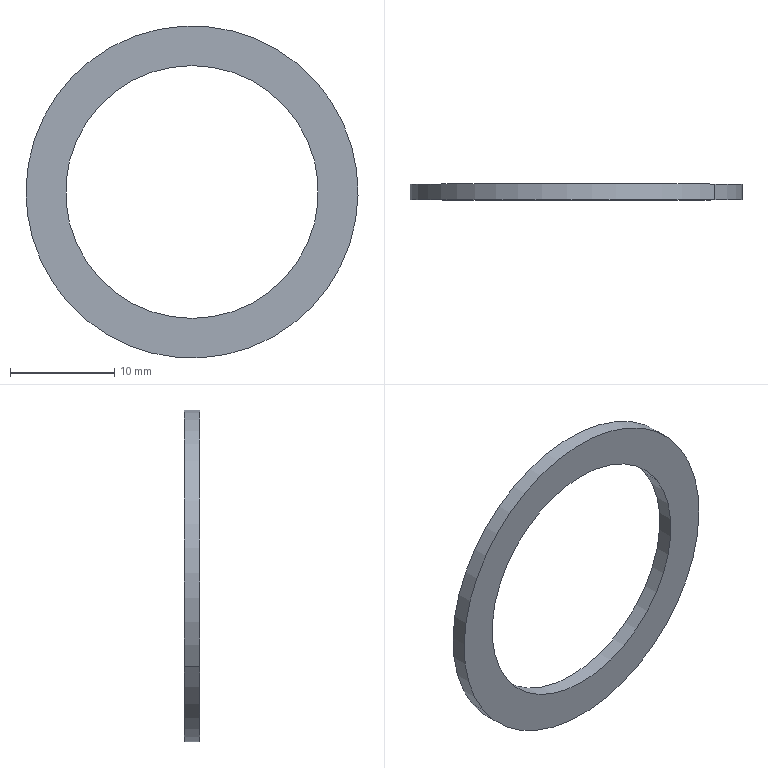Part | SolidWorks | features BaseBody 1 | 1 solid | 6 faces | box 31.8 x 1.5 x 31.8 mm | volume 501.398 mm3 | cylinder 4 | plane 2 | commonest cylinder face diameters 24.2 x2 31.8 x2
STEP:
#1=CARTESIAN_POINT('',(196.311,-137.,298.196));
#2=VERTEX_POINT('',#1);
#3=CARTESIAN_POINT('',(169.689,-137.,280.804));
#4=VERTEX_POINT('',#3);
#5=CARTESIAN_POINT('',(183.,-137.,289.5));
#6=DIRECTION('',(0.,-1.,0.));
#7=DIRECTION('',(0.,0.,1.));
#8=AXIS2_PLACEMENT_3D('',#5,#6,#7);
#9=CIRCLE('',#8,15.9);
#10=EDGE_CURVE('',#2,#4,#9,.T.);
#11=ORIENTED_EDGE('',*,*,#10,.F.);
#12=CARTESIAN_POINT('',(196.311,-135.5,298.196));
#13=VERTEX_POINT('',#12);
#14=CARTESIAN_POINT('',(196.311,-137.,298.196));
#15=DIRECTION('',(0.,1.,0.));
#16=VECTOR('',#15,1000.);
#17=LINE('',#14,#16);
#18=EDGE_CURVE('',#2,#13,#17,.T.);
#19=ORIENTED_EDGE('',*,*,#18,.T.);
#20=CARTESIAN_POINT('',(169.689,-135.5,280.804));
#21=VERTEX_POINT('',#20);
#22=CARTESIAN_POINT('',(183.,-135.5,289.5));
#23=DIRECTION('',(0.,1.,0.));
#24=DIRECTION('',(0.,0.,1.));
#25=AXIS2_PLACEMENT_3D('',#22,#23,#24);
#26=CIRCLE('',#25,15.9);
#27=EDGE_CURVE('',#21,#13,#26,.T.);
#28=ORIENTED_EDGE('',*,*,#27,.F.);
#29=CARTESIAN_POINT('',(169.689,-137.,280.804));
#30=DIRECTION('',(0.,1.,0.));
#31=VECTOR('',#30,1000.);
#32=LINE('',#29,#31);
#33=EDGE_CURVE('',#4,#21,#32,.T.);
#34=ORIENTED_EDGE('',*,*,#33,.F.);
#35=EDGE_LOOP('',(#11,#19,#28,#34));
#36=FACE_OUTER_BOUND('',#35,.T.);
#37=CARTESIAN_POINT('',(183.,-137.,289.5));
#38=DIRECTION('',(0.,1.,0.));
#39=DIRECTION('',(-0.8372,0.,-0.5469));
#40=AXIS2_PLACEMENT_3D('',#37,#38,#39);
#41=CYLINDRICAL_SURFACE('',#40,15.9);
#42=ADVANCED_FACE('',(#36),#41,.T.);
#43=CARTESIAN_POINT('',(172.87,-137.,282.882));
#44=VERTEX_POINT('',#43);
#45=CARTESIAN_POINT('',(193.13,-137.,296.118));
#46=VERTEX_POINT('',#45);
#47=CARTESIAN_POINT('',(183.,-137.,289.5));
#48=DIRECTION('',(0.,-1.,0.));
#49=DIRECTION('',(0.,0.,1.));
#50=AXIS2_PLACEMENT_3D('',#47,#48,#49);
#51=CIRCLE('',#50,12.1);
#52=EDGE_CURVE('',#44,#46,#51,.T.);
#53=ORIENTED_EDGE('',*,*,#52,.T.);
#54=CARTESIAN_POINT('',(193.13,-135.5,296.118));
#55=VERTEX_POINT('',#54);
#56=CARTESIAN_POINT('',(193.13,-137.,296.118));
#57=DIRECTION('',(0.,1.,0.));
#58=VECTOR('',#57,1000.);
#59=LINE('',#56,#58);
#60=EDGE_CURVE('',#46,#55,#59,.T.);
#61=ORIENTED_EDGE('',*,*,#60,.T.);
#62=CARTESIAN_POINT('',(172.87,-135.5,282.882));
#63=VERTEX_POINT('',#62);
#64=CARTESIAN_POINT('',(183.,-135.5,289.5));
#65=DIRECTION('',(0.,-1.,0.));
#66=DIRECTION('',(0.,0.,1.));
#67=AXIS2_PLACEMENT_3D('',#64,#65,#66);
#68=CIRCLE('',#67,12.1);
#69=EDGE_CURVE('',#63,#55,#68,.T.);
#70=ORIENTED_EDGE('',*,*,#69,.F.);
#71=CARTESIAN_POINT('',(172.87,-137.,282.882));
#72=DIRECTION('',(0.,1.,0.));
#73=VECTOR('',#72,1000.);
#74=LINE('',#71,#73);
#75=EDGE_CURVE('',#44,#63,#74,.T.);
#76=ORIENTED_EDGE('',*,*,#75,.F.);
#77=EDGE_LOOP('',(#53,#61,#70,#76));
#78=FACE_OUTER_BOUND('',#77,.T.);
#79=CARTESIAN_POINT('',(183.,-137.,289.5));
#80=DIRECTION('',(0.,1.,0.));
#81=DIRECTION('',(-0.8372,0.,-0.5469));
#82=AXIS2_PLACEMENT_3D('',#79,#80,#81);
#83=CYLINDRICAL_SURFACE('',#82,12.1);
#84=ADVANCED_FACE('',(#78),#83,.F.);
#85=ORIENTED_EDGE('',*,*,#27,.T.);
#86=CARTESIAN_POINT('',(183.,-135.5,289.5));
#87=DIRECTION('',(0.,1.,0.));
#88=DIRECTION('',(0.,0.,1.));
#89=AXIS2_PLACEMENT_3D('',#86,#87,#88);
#90=CIRCLE('',#89,15.9);
#91=EDGE_CURVE('',#13,#21,#90,.T.);
#92=ORIENTED_EDGE('',*,*,#91,.T.);
#93=EDGE_LOOP('',(#85,#92));
#94=FACE_OUTER_BOUND('',#93,.T.);
#95=ORIENTED_EDGE('',*,*,#69,.T.);
#96=CARTESIAN_POINT('',(183.,-135.5,289.5));
#97=DIRECTION('',(0.,-1.,0.));
#98=DIRECTION('',(0.,0.,1.));
#99=AXIS2_PLACEMENT_3D('',#96,#97,#98);
#100=CIRCLE('',#99,12.1);
#101=EDGE_CURVE('',#55,#63,#100,.T.);
#102=ORIENTED_EDGE('',*,*,#101,.T.);
#103=EDGE_LOOP('',(#95,#102));
#104=FACE_BOUND('',#103,.T.);
#105=CARTESIAN_POINT('',(176.382,-135.5,299.63));
#106=DIRECTION('',(0.,1.,0.));
#107=DIRECTION('',(0.,0.,-1.));
#108=AXIS2_PLACEMENT_3D('',#105,#106,#107);
#109=PLANE('',#108);
#110=ADVANCED_FACE('',(#94,#104),#109,.T.);
#111=ORIENTED_EDGE('',*,*,#60,.F.);
#112=CARTESIAN_POINT('',(183.,-137.,289.5));
#113=DIRECTION('',(0.,-1.,0.));
#114=DIRECTION('',(0.,0.,1.));
#115=AXIS2_PLACEMENT_3D('',#112,#113,#114);
#116=CIRCLE('',#115,12.1);
#117=EDGE_CURVE('',#46,#44,#116,.T.);
#118=ORIENTED_EDGE('',*,*,#117,.T.);
#119=ORIENTED_EDGE('',*,*,#75,.T.);
#120=ORIENTED_EDGE('',*,*,#101,.F.);
#121=EDGE_LOOP('',(#111,#118,#119,#120));
#122=FACE_OUTER_BOUND('',#121,.T.);
#123=CARTESIAN_POINT('',(183.,-137.,289.5));
#124=DIRECTION('',(0.,1.,0.));
#125=DIRECTION('',(-0.8372,0.,-0.5469));
#126=AXIS2_PLACEMENT_3D('',#123,#124,#125);
#127=CYLINDRICAL_SURFACE('',#126,12.1);
#128=ADVANCED_FACE('',(#122),#127,.F.);
#129=ORIENTED_EDGE('',*,*,#18,.F.);
#130=CARTESIAN_POINT('',(183.,-137.,289.5));
#131=DIRECTION('',(0.,-1.,0.));
#132=DIRECTION('',(0.,0.,1.));
#133=AXIS2_PLACEMENT_3D('',#130,#131,#132);
#134=CIRCLE('',#133,15.9);
#135=EDGE_CURVE('',#4,#2,#134,.T.);
#136=ORIENTED_EDGE('',*,*,#135,.F.);
#137=ORIENTED_EDGE('',*,*,#33,.T.);
#138=ORIENTED_EDGE('',*,*,#91,.F.);
#139=EDGE_LOOP('',(#129,#136,#137,#138));
#140=FACE_OUTER_BOUND('',#139,.T.);
#141=CARTESIAN_POINT('',(183.,-137.,289.5));
#142=DIRECTION('',(0.,1.,0.));
#143=DIRECTION('',(-0.8372,0.,-0.5469));
#144=AXIS2_PLACEMENT_3D('',#141,#142,#143);
#145=CYLINDRICAL_SURFACE('',#144,15.9);
#146=ADVANCED_FACE('',(#140),#145,.T.);
#147=ORIENTED_EDGE('',*,*,#135,.T.);
#148=ORIENTED_EDGE('',*,*,#10,.T.);
#149=EDGE_LOOP('',(#147,#148));
#150=FACE_OUTER_BOUND('',#149,.T.);
#151=ORIENTED_EDGE('',*,*,#52,.F.);
#152=ORIENTED_EDGE('',*,*,#117,.F.);
#153=EDGE_LOOP('',(#151,#152));
#154=FACE_BOUND('',#153,.T.);
#155=CARTESIAN_POINT('',(174.304,-137.,302.811));
#156=DIRECTION('',(0.,1.,0.));
#157=DIRECTION('',(0.,0.,-1.));
#158=AXIS2_PLACEMENT_3D('',#155,#156,#157);
#159=PLANE('',#158);
#160=ADVANCED_FACE('',(#150,#154),#159,.F.);
#161=CLOSED_SHELL('',(#42,#84,#110,#128,#146,#160));
#162=MANIFOLD_SOLID_BREP('',#161);
#163=CARTESIAN_POINT('',(0.,0.,0.));
#164=DIRECTION('',(0.,0.,1.));
#165=DIRECTION('',(1.,0.,0.));
#166=AXIS2_PLACEMENT_3D('',#163,#164,#165);
#167=(LENGTH_UNIT()NAMED_UNIT(*)SI_UNIT(.MILLI.,.METRE.));
#168=UNCERTAINTY_MEASURE_WITH_UNIT(LENGTH_MEASURE(0.00001),#167,'','');
#169=(NAMED_UNIT(*)PLANE_ANGLE_UNIT()SI_UNIT($,.RADIAN.));
#170=(NAMED_UNIT(*)SI_UNIT($,.STERADIAN.)SOLID_ANGLE_UNIT());
#171=(GEOMETRIC_REPRESENTATION_CONTEXT(3)GLOBAL_UNCERTAINTY_ASSIGNED_CONTEXT((#168))GLOBAL_UNIT_ASSIGNED_CONTEXT((#167,#169,#170))REPRESENTATION_CONTEXT('',''));
#172=ADVANCED_BREP_SHAPE_REPRESENTATION('',(#162,#166),#171);